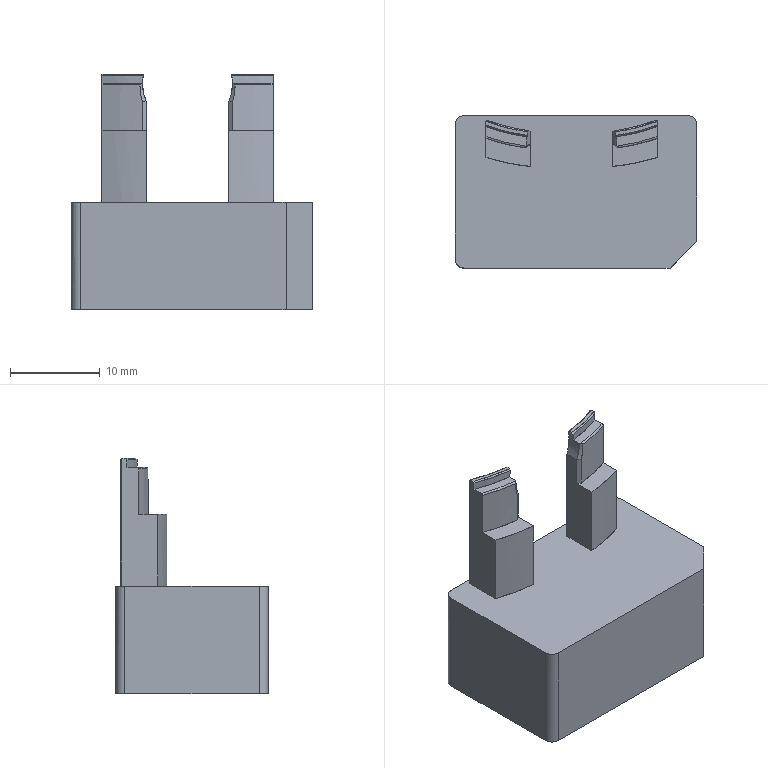NC program | PowerMill | posted by the shop | part box 27 x 17 x 26.255 mm
Lines 17311 to 19049 of 169183:
( TOOL ID   D3_1_1 )
( TOOL DIA. 3. TIP RAD 0 LENGTH 69.4 )
( Z = -14.42 )
T10 M6
T13
G91 G28 Z0
G0 G90 G54
M08
S18000 M3
X0 Y0 M8
G43 Z10.805 H10
X7.533 Y9.349
Z.915
G1 Z-.285 F1200
X7.55 Y9.308 F2000
X7.57 Y9.27
X7.594 Y9.233
X7.621 Y9.199
X7.651 Y9.167
X7.684 Y9.138
X7.72 Y9.112
X7.757 Y9.09
X7.797 Y9.071
X7.838 Y9.056
X7.88 Y9.044
X7.923 Y9.037
X7.966 Y9.033
X8.01
X8.054 Y9.038
X8.097 Y9.046
X8.139 Y9.058
X8.148 Y9.061
X8.39 Y9.149
X8.548 Y9.208
X8.619 Y9.233
X8.691 Y9.254
X8.764 Y9.271
X8.839 Y9.285
X8.913 Y9.294
X8.989 Y9.299
X9.064 Y9.301
X9.139 Y9.298
X9.214 Y9.291
X9.289 Y9.281
X9.363 Y9.266
X9.436 Y9.248
X9.508 Y9.225
X9.579 Y9.199
X9.648 Y9.169
X9.716 Y9.136
X9.782 Y9.099
X9.846 Y9.059
X9.907 Y9.015
X9.966 Y8.968
X10.022 Y8.919
X10.076 Y8.866
X10.127 Y8.81
X10.175 Y8.752
X10.22 Y8.691
X10.261 Y8.628
X10.3 Y8.563
X10.334 Y8.496
X10.365 Y8.427
X10.393 Y8.357
X10.416 Y8.286
X10.436 Y8.213
X10.452 Y8.14
X10.464 Y8.065
X10.472 Y7.991
X10.475 Y7.937
X10.477 Y7.883
Y7.829
X10.478 Y7.775
Y7.717
Y7.638
Y7.584
X10.477 Y7.523
Y7.469
X10.476 Y7.415
X10.475 Y7.361
X10.473 Y7.307
X10.467 Y7.234
X10.456 Y7.162
X10.442 Y7.089
X10.424 Y7.017
X10.401 Y6.945
X10.375 Y6.875
X10.345 Y6.806
X10.312 Y6.738
X10.275 Y6.672
X10.235 Y6.609
X10.191 Y6.547
X10.144 Y6.488
X10.094 Y6.432
X10.041 Y6.378
X9.985 Y6.327
X9.927 Y6.279
X9.866 Y6.234
X9.803 Y6.193
X9.738 Y6.155
X9.671 Y6.12
X9.603 Y6.089
X9.532 Y6.062
X9.26 Y5.963
X8.986 Y5.868
X8.711 Y5.776
X8.435 Y5.688
X8.158 Y5.604
X7.874 Y5.521
X7.589 Y5.443
X7.303 Y5.368
X7.016 Y5.297
X6.729 Y5.229
X6.434 Y5.164
X6.137 Y5.103
X5.838 Y5.046
X5.55 Y4.994
X5.257 Y4.945
X4.946 Y4.897
X4.649 Y4.855
X4.574 Y4.846
X4.498 Y4.841
X4.423 Y4.839
X4.352 Y4.841
X4.282 Y4.846
X4.211 Y4.855
X4.137 Y4.869
X4.064 Y4.886
X3.992 Y4.907
X3.921 Y4.932
X3.851 Y4.961
X3.783 Y4.993
X3.717 Y5.029
X3.652 Y5.068
X3.59 Y5.111
X3.53 Y5.157
X3.473 Y5.206
X3.418 Y5.258
X3.366 Y5.313
X3.317 Y5.37
X3.271 Y5.43
X3.231 Y5.489
X3.193 Y5.552
X3.158 Y5.617
X3.126 Y5.685
X3.097 Y5.757
X3.07 Y5.831
X3.049 Y5.901
X3.032 Y5.971
X3.018 Y6.043
X3.008 Y6.115
X3.002 Y6.186
X2.999 Y6.271
X2.998 Y6.377
Y6.498
X2.999 Y6.683
X3. Y6.748
X3.003 Y6.81
X3.009 Y6.875
X3.021 Y6.945
X3.037 Y7.02
X3.056 Y7.097
X3.079 Y7.171
X3.105 Y7.241
X3.134 Y7.308
X3.166 Y7.373
X3.203 Y7.439
X3.244 Y7.502
X3.288 Y7.564
X3.335 Y7.623
X3.385 Y7.68
X3.438 Y7.734
X3.494 Y7.785
X3.552 Y7.833
X3.612 Y7.877
X3.674 Y7.918
X3.739 Y7.956
X3.805 Y7.991
X3.873 Y8.021
X3.943 Y8.049
X4.015 Y8.073
X4.089 Y8.093
X4.164 Y8.109
X4.241 Y8.122
X4.319 Y8.133
X4.575 Y8.17
X4.849 Y8.214
X5.118 Y8.26
X5.397 Y8.313
X5.664 Y8.367
X5.933 Y8.425
X6.204 Y8.487
X6.472 Y8.553
X6.737 Y8.622
X7.001 Y8.695
X7.265 Y8.772
X7.527 Y8.853
X7.787 Y8.938
X8.046 Y9.026
X8.148 Y9.061
X8.189 Y9.078
X8.228 Y9.098
X8.264 Y9.121
X8.299 Y9.148
X8.331 Y9.178
X8.36 Y9.21
X8.387 Y9.245
X8.409 Y9.283
X8.429 Y9.322
X8.444 Y9.363
X8.456 Y9.405
X8.464 Y9.448
X8.468 Y9.492
Y9.535
X8.464 Y9.579
X8.457 Y9.622
X8.445 Y9.664
X8.442 Y9.673
X7.528 Y9.371 Z-.305
X7.545 Y9.331
X7.565 Y9.292
X7.588 Y9.255
X7.615 Y9.221
X7.645 Y9.189
X7.678 Y9.16
X7.713 Y9.134
X7.75 Y9.111
X7.79 Y9.092
X7.831 Y9.076
X7.873 Y9.065
X7.916 Y9.057
X7.96 Y9.053
X8.003
X8.047 Y9.057
X8.09 Y9.065
X8.132 Y9.077
X8.141 Y9.08
X8.27 Y9.126
X8.348 Y9.155
X8.396 Y9.172
X8.443 Y9.19
X8.491 Y9.209
X8.539 Y9.227
X8.588 Y9.244
X8.636 Y9.26
X8.685 Y9.273
X8.735 Y9.285
X8.785 Y9.296
X8.858 Y9.308
X8.933 Y9.316
X9.008 Y9.32
X9.083
X9.158 Y9.317
X9.233 Y9.309
X9.308 Y9.297
X9.381 Y9.281
X9.454 Y9.262
X9.526 Y9.238
X9.596 Y9.211
X9.665 Y9.181
X9.731 Y9.146
X9.796 Y9.109
X9.859 Y9.067
X9.92 Y9.023
X9.979 Y8.975
X10.034 Y8.925
X10.088 Y8.871
X10.138 Y8.815
X10.185 Y8.756
X10.229 Y8.694
X10.269 Y8.631
X10.306 Y8.565
X10.34 Y8.498
X10.37 Y8.429
X10.396 Y8.359
X10.419 Y8.287
X10.438 Y8.214
X10.453 Y8.138
X10.465 Y8.061
X10.472 Y7.99
X10.476 Y7.912
X10.477 Y7.824
Y7.448
Y7.358
X10.475 Y7.294
X10.47 Y7.24
X10.463 Y7.184
X10.454 Y7.127
X10.438 Y7.052
X10.418 Y6.979
X10.395 Y6.907
X10.368 Y6.837
X10.338 Y6.769
X10.304 Y6.701
X10.266 Y6.636
X10.225 Y6.573
X10.18 Y6.512
X10.133 Y6.453
X10.082 Y6.397
X10.028 Y6.344
X9.972 Y6.294
X9.913 Y6.247
X9.852 Y6.203
X9.788 Y6.162
X9.723 Y6.125
X9.656 Y6.091
X9.588 Y6.062
X9.52 Y6.036
X9.248 Y5.937
X8.973 Y5.842
X8.693 Y5.749
X8.418 Y5.661
X8.141 Y5.577
X7.857 Y5.496
X7.567 Y5.416
X7.303 Y5.347
X7.038 Y5.281
X6.745 Y5.213
X6.451 Y5.148
X6.155 Y5.086
X5.857 Y5.029
X5.557 Y4.975
X5.256 Y4.925
X4.952 Y4.878
X4.707 Y4.843
X4.637 Y4.834
X4.567 Y4.826
X4.496 Y4.821
X4.425 Y4.819
X4.353 Y4.821
X4.279 Y4.827
X4.205 Y4.837
X4.133 Y4.851
X4.061 Y4.868
X3.99 Y4.889
X3.92 Y4.913
X3.851 Y4.942
X3.783 Y4.974
X3.717 Y5.01
X3.653 Y5.05
X3.591 Y5.093
X3.531 Y5.14
X3.473 Y5.189
X3.419 Y5.241
X3.367 Y5.296
X3.319 Y5.354
X3.273 Y5.413
X3.232 Y5.475
X3.193 Y5.539
X3.158 Y5.605
X3.125 Y5.674
X3.097 Y5.743
X3.073 Y5.811
X3.053 Y5.879
X3.038 Y5.946
X3.024 Y6.013
X3.016 Y6.059
X3.01 Y6.106
X3.004 Y6.158
X3. Y6.205
X2.999 Y6.252
X2.998 Y6.648
X3. Y6.736
X3.004 Y6.812
X3.009 Y6.862
X3.016 Y6.912
X3.025 Y6.961
X3.034 Y7.011
X3.045 Y7.06
X3.064 Y7.132
X3.088 Y7.204
X3.115 Y7.275
X3.145 Y7.344
X3.18 Y7.411
X3.217 Y7.476
X3.259 Y7.539
X3.303 Y7.6
X3.351 Y7.658
X3.401 Y7.714
X3.455 Y7.768
X3.511 Y7.818
X3.57 Y7.865
X3.632 Y7.909
X3.695 Y7.949
X3.76 Y7.987
X3.827 Y8.02
X3.896 Y8.05
X3.967 Y8.076
X4.039 Y8.099
X4.113 Y8.118
X4.188 Y8.134
X4.265 Y8.145
X4.531 Y8.184
X4.812 Y8.228
X5.092 Y8.276
X5.368 Y8.327
X5.642 Y8.382
X5.916 Y8.441
X6.189 Y8.504
X6.458 Y8.57
X6.726 Y8.64
X6.992 Y8.714
X7.248 Y8.788
X7.49 Y8.863
X7.754 Y8.947
X7.883 Y8.991
X8.012 Y9.035
X8.141 Y9.08
X8.182 Y9.097
X8.221 Y9.117
X8.257 Y9.141
X8.292 Y9.167
X8.324 Y9.197
X8.353 Y9.23
X8.379 Y9.265
X8.402 Y9.303
X8.421 Y9.342
X8.437 Y9.383
X8.448 Y9.425
X8.456 Y9.468
X8.46 Y9.512
Y9.555
X8.456 Y9.599
X8.448 Y9.642
X8.436 Y9.684
X8.433 Y9.693
X7.522 Y9.393 Z-.325
X7.539 Y9.352
X7.559 Y9.313
X7.582 Y9.276
X7.609 Y9.242
X7.639 Y9.21
X7.671 Y9.18
X7.706 Y9.154
X7.744 Y9.132
X7.783 Y9.112
X7.824 Y9.097
X7.866 Y9.085
X7.909 Y9.077
X7.953 Y9.073
X7.996
X8.04 Y9.077
X8.083 Y9.085
X8.125 Y9.096
X8.134 Y9.1
X8.217 Y9.129
X8.269 Y9.147
X8.314 Y9.164
X8.358 Y9.18
X8.403 Y9.197
X8.447 Y9.213
X8.492 Y9.23
X8.536 Y9.247
X8.582 Y9.263
X8.638 Y9.281
X8.689 Y9.295
X8.735 Y9.306
X8.781 Y9.315
X8.828 Y9.323
X8.875 Y9.329
X8.948 Y9.336
X9.022 Y9.34
X9.096 Y9.339
X9.171 Y9.334
X9.246 Y9.325
X9.32 Y9.312
X9.394 Y9.295
X9.467 Y9.275
X9.538 Y9.25
X9.608 Y9.222
X9.676 Y9.19
X9.743 Y9.155
X9.807 Y9.116
X9.87 Y9.074
X9.93 Y9.029
X9.988 Y8.98
X10.043 Y8.928
X10.095 Y8.874
X10.144 Y8.817
X10.191 Y8.757
X10.234 Y8.696
X10.273 Y8.632
X10.309 Y8.565
X10.343 Y8.496
X10.372 Y8.425
X10.399 Y8.352
X10.421 Y8.278
X10.44 Y8.202
X10.455 Y8.129
X10.466 Y8.055
X10.473 Y7.98
X10.476 Y7.899
X10.477 Y7.814
Y7.348
X10.475 Y7.278
X10.469 Y7.206
X10.459 Y7.133
X10.444 Y7.059
X10.427 Y6.986
X10.405 Y6.913
X10.379 Y6.843
X10.35 Y6.773
X10.317 Y6.705
X10.281 Y6.639
X10.241 Y6.575
X10.198 Y6.513
X10.151 Y6.454
X10.102 Y6.397
X10.049 Y6.343
X9.994 Y6.291
X9.936 Y6.243
X9.876 Y6.198
X9.813 Y6.156
X9.748 Y6.117
X9.681 Y6.082
X9.613 Y6.051
X9.542 Y6.023
X9.265 Y5.922
X8.986 Y5.825
X8.705 Y5.732
X8.421 Y5.642
X8.137 Y5.555
X7.85 Y5.473
X7.561 Y5.394
X7.271 Y5.318
X6.978 Y5.246
X6.684 Y5.178
X6.388 Y5.114
X6.091 Y5.053
X5.791 Y4.996
X5.491 Y4.943
X5.189 Y4.894
X4.927 Y4.854
X4.649 Y4.815
X4.571 Y4.806
X4.494 Y4.801
X4.417 Y4.8
X4.341 Y4.803
X4.266 Y4.81
X4.192 Y4.82
X4.118 Y4.835
X4.046 Y4.854
X3.974 Y4.876
X3.903 Y4.902
X3.834 Y4.932
X3.766 Y4.966
X3.701 Y5.003
X3.637 Y5.044
X3.576 Y5.087
X3.517 Y5.135
X3.46 Y5.185
X3.407 Y5.238
X3.356 Y5.293
X3.308 Y5.352
X3.264 Y5.413
X3.223 Y5.475
X3.185 Y5.54
X3.151 Y5.607
X3.12 Y5.676
X3.092 Y5.747
X3.069 Y5.82
X3.049 Y5.893
X3.032 Y5.968
X3.017 Y6.054
X3.007 Y6.13
X3.001 Y6.198
X2.999 Y6.262
Y6.337
X2.998 Y6.412
Y6.487
Y6.562
Y6.636
X2.999 Y6.711
X3.001 Y6.774
X3.006 Y6.839
X3.016 Y6.911
X3.031 Y6.996
X3.046 Y7.067
X3.064 Y7.138
X3.085 Y7.208
X3.111 Y7.278
X3.141 Y7.347
X3.174 Y7.415
X3.211 Y7.48
X3.252 Y7.544
X3.295 Y7.606
X3.342 Y7.665
X3.392 Y7.721
X3.445 Y7.775
X3.5 Y7.826
X3.559 Y7.874
X3.619 Y7.919
X3.682 Y7.96
X3.747 Y7.998
X3.814 Y8.032
X3.882 Y8.063
X3.953 Y8.091
X4.024 Y8.115
X4.098 Y8.135
X4.172 Y8.151
X4.248 Y8.163
X4.324 Y8.174
X4.598 Y8.214
X4.881 Y8.26
X5.16 Y8.309
X5.434 Y8.361
X5.708 Y8.417
X5.981 Y8.476
X6.253 Y8.54
X6.522 Y8.607
X6.789 Y8.678
X7.054 Y8.752
X7.317 Y8.83
X7.555 Y8.904
X7.759 Y8.97
X7.964 Y9.04
X8.134 Y9.1
X8.175 Y9.116
X8.214 Y9.136
X8.251 Y9.16
X8.285 Y9.186
X8.318 Y9.216
X8.347 Y9.249
X8.373 Y9.284
X8.396 Y9.321
X8.415 Y9.36
X8.431 Y9.401
X8.442 Y9.443
X8.45 Y9.486
X8.454 Y9.53
Y9.574
X8.45 Y9.617
X8.443 Y9.66
X8.431 Y9.703
X8.428 Y9.712
X7.512 Y9.406 Z-.345
X7.529 Y9.365
X7.549 Y9.327
X7.573 Y9.29
X7.6 Y9.256
X7.631 Y9.224
X7.663 Y9.195
X7.699 Y9.169
X7.736 Y9.147
X7.776 Y9.128
X7.817 Y9.113
X7.859 Y9.101
X7.902 Y9.094
X7.946 Y9.09
X7.99 Y9.091
X8.033 Y9.095
X8.076 Y9.104
X8.118 Y9.116
X8.127 Y9.119
X8.136 Y9.122
X8.189 Y9.141
X8.241 Y9.16
X8.294 Y9.179
X8.347 Y9.197
X8.348 Y9.198
X8.401 Y9.217
X8.467 Y9.241
X8.515 Y9.26
X8.574 Y9.281
X8.625 Y9.297
X8.674 Y9.311
X8.723 Y9.323
X8.773 Y9.333
X8.823 Y9.341
X8.874 Y9.348
X8.942 Y9.354
X9.014 Y9.357
X9.088 Y9.356
X9.163 Y9.351
X9.238 Y9.342
X9.312 Y9.329
X9.385 Y9.312
X9.458 Y9.291
X9.529 Y9.267
X9.599 Y9.239
X9.667 Y9.207
X9.734 Y9.171
X9.799 Y9.132
X9.861 Y9.09
X9.921 Y9.044
X9.979 Y8.996
X10.034 Y8.944
X10.086 Y8.89
X10.135 Y8.833
X10.182 Y8.771
X10.226 Y8.708
X10.267 Y8.642
X10.305 Y8.574
X10.339 Y8.504
X10.37 Y8.432
X10.397 Y8.358
X10.42 Y8.284
X10.439 Y8.208
X10.454 Y8.136
X10.465 Y8.064
X10.472 Y7.989
X10.476 Y7.912
X10.477 Y7.838
Y7.353
X10.476 Y7.278
X10.47 Y7.202
X10.461 Y7.127
X10.448 Y7.053
X10.43 Y6.979
X10.409 Y6.906
X10.385 Y6.835
X10.356 Y6.765
X10.324 Y6.697
X10.288 Y6.631
X10.249 Y6.566
X10.206 Y6.504
X10.16 Y6.444
X10.112 Y6.387
X10.06 Y6.332
X10.005 Y6.28
X9.948 Y6.231
X9.888 Y6.185
X9.825 Y6.143
X9.761 Y6.103
X9.695 Y6.068
X9.626 Y6.035
X9.557 Y6.007
X9.486 Y5.981
X9.209 Y5.881
X8.929 Y5.785
X8.648 Y5.692
X8.364 Y5.603
X8.078 Y5.518
X7.792 Y5.436
X7.503 Y5.358
X7.212 Y5.283
X6.918 Y5.212
X6.627 Y5.145
X6.332 Y5.082
X6.034 Y5.022
X5.731 Y4.965
X5.455 Y4.917
X5.165 Y4.87
X4.849 Y4.823
X4.649 Y4.795
X4.57 Y4.786
X4.493 Y4.781
X4.416 Y4.78
X4.339 Y4.784
X4.264 Y4.791
X4.19 Y4.802
X4.118 Y4.816
X4.046 Y4.835
X3.974 Y4.858
X3.903 Y4.884
X3.834 Y4.914
X3.767 Y4.948
X3.701 Y4.986
X3.637 Y5.027
X3.576 Y5.071
X3.517 Y5.118
X3.461 Y5.168
X3.407 Y5.221
X3.357 Y5.277
X3.31 Y5.334
X3.266 Y5.395
X3.225 Y5.458
X3.186 Y5.525
X3.15 Y5.595
X3.123 Y5.655
X3.099 Y5.719
X3.077 Y5.788
X3.056 Y5.865
X3.037 Y5.948
X3.02 Y6.029
X3.011 Y6.089
X3.005 Y6.14
X3.003 Y6.189
X2.999 Y6.297
X2.998 Y6.394
Y6.498
Y6.617
Y6.704
X3.002 Y6.78
X3.009 Y6.863
X3.021 Y6.947
X3.037 Y7.03
X3.056 Y7.113
X3.076 Y7.186
X3.097 Y7.252
X3.124 Y7.321
X3.154 Y7.389
X3.188 Y7.455
X3.225 Y7.517
X3.264 Y7.578
X3.31 Y7.64
X3.359 Y7.7
X3.409 Y7.756
X3.463 Y7.809
X3.518 Y7.859
X3.576 Y7.905
X3.636 Y7.948
X3.7 Y7.99
X3.766 Y8.027
X3.834 Y8.061
X3.903 Y8.091
X3.974 Y8.118
X4.045 Y8.14
X4.11 Y8.157
X4.175 Y8.171
X4.241 Y8.182
X4.307 Y8.192
X4.373 Y8.201
X4.439 Y8.211
X4.505 Y8.22
X4.571 Y8.23
X4.637 Y8.241
X4.703 Y8.251
X4.988 Y8.298
X5.264 Y8.348
X5.531 Y8.4
X5.796 Y8.456
X6.07 Y8.517
X6.341 Y8.582
X6.605 Y8.649
X6.868 Y8.72
X7.13 Y8.795
X7.398 Y8.876
X7.575 Y8.932
X7.796 Y9.003
X7.849 Y9.02
X7.902 Y9.038
X7.955 Y9.056
X8.007 Y9.075
X8.061 Y9.095
X8.127 Y9.119
X8.168 Y9.136
X8.206 Y9.156
X8.243 Y9.18
X8.278 Y9.207
X8.309 Y9.237
X8.338 Y9.27
X8.364 Y9.306
X8.386 Y9.343
X8.405 Y9.383
X8.42 Y9.424
X8.432 Y9.466
X8.439 Y9.509
X8.443 Y9.553
X8.442 Y9.596
X8.438 Y9.64
X8.43 Y9.683
X8.418 Y9.725
X8.414 Y9.734
X7.507 Y9.428 Z-.365
X7.524 Y9.387
X7.544 Y9.348
X7.568 Y9.311
X7.595 Y9.277
X7.625 Y9.245
X7.658 Y9.216
X7.693 Y9.19
X7.73 Y9.167
X7.77 Y9.148
X7.81 Y9.133
X7.853 Y9.121
X7.896 Y9.113
X7.939 Y9.109
X7.983 Y9.11
X8.027 Y9.114
X8.07 Y9.122
X8.112 Y9.134
X8.121 Y9.137
X8.248 Y9.182
X8.348 Y9.219
X8.483 Y9.269
X8.574 Y9.301
X8.651 Y9.324
X8.719 Y9.342
X8.783 Y9.355
X8.842 Y9.363
X8.903 Y9.369
X8.981 Y9.372
X9.059 Y9.371
X9.137 Y9.367
X9.214 Y9.358
X9.287 Y9.347
X9.359 Y9.331
X9.43 Y9.311
X9.501 Y9.288
X9.57 Y9.261
X9.639 Y9.23
X9.705 Y9.195
X9.77 Y9.157
X9.833 Y9.115
X9.894 Y9.07
X9.953 Y9.021
X10.01 Y8.968
X10.065 Y8.913
X10.117 Y8.854
X10.166 Y8.793
X10.212 Y8.73
X10.254 Y8.664
X10.293 Y8.597
X10.328 Y8.527
X10.36 Y8.456
X10.388 Y8.383
X10.412 Y8.309
X10.433 Y8.234
X10.447 Y8.171
X10.46 Y8.097
X10.469 Y8.03
X10.473 Y7.969
X10.474 Y7.909
X10.477 Y7.638
X10.478 Y7.348
X10.476 Y7.265
X10.47 Y7.186
X10.462 Y7.112
X10.45 Y7.041
X10.433 Y6.967
X10.412 Y6.895
X10.388 Y6.823
X10.36 Y6.753
X10.328 Y6.685
X10.293 Y6.618
X10.254 Y6.553
X10.212 Y6.491
X10.167 Y6.43
X10.118 Y6.373
X10.067 Y6.318
X10.012 Y6.265
X9.955 Y6.216
X9.896 Y6.17
X9.834 Y6.127
X9.77 Y6.087
X9.703 Y6.051
X9.636 Y6.018
X9.566 Y5.989
X9.495 Y5.963
X9.219 Y5.863
X8.94 Y5.767
X8.658 Y5.675
X8.374 Y5.585
X8.088 Y5.5
X7.801 Y5.418
X7.512 Y5.339
X7.221 Y5.265
X6.928 Y5.193
X6.633 Y5.126
X6.337 Y5.062
X6.038 Y5.002
X5.74 Y4.946
X5.439 Y4.894
X5.154 Y4.848
X4.848 Y4.802
X4.649 Y4.775
X4.571 Y4.766
X4.494 Y4.761
X4.417
X4.342 Y4.764
X4.268 Y4.771
X4.195 Y4.782
X4.121 Y4.797
X4.048 Y4.816
X3.976 Y4.839
X3.905 Y4.865
X3.836 Y4.896
X3.769 Y4.93
X3.703 Y4.967
X3.64 Y5.008
X3.579 Y5.052
X3.52 Y5.099
X3.464 Y5.149
X3.41 Y5.203
X3.36 Y5.259
X3.312 Y5.318
X3.269 Y5.377
X3.228 Y5.439
X3.19 Y5.505
X3.154 Y5.575
X3.128 Y5.633
X3.104 Y5.695
X3.082 Y5.764
X3.059 Y5.845
X3.049 Y5.886
X3.042 Y5.919
X3.035 Y5.953
X3.028 Y5.988
X3.018 Y6.043
X3.013 Y6.077
X3.009 Y6.11
X3.005 Y6.144
X3.003 Y6.179
X2.999 Y6.288
X2.998 Y6.385
Y6.609
X2.999 Y6.733
X3.002 Y6.791
X3.008 Y6.855
X3.019 Y6.929
X3.037 Y7.029
X3.052 Y7.104
X3.071 Y7.178
X3.093 Y7.249
X3.119 Y7.32
X3.149 Y7.388
X3.182 Y7.456
X3.219 Y7.522
X3.259 Y7.586
X3.303 Y7.647
X3.35 Y7.706
X3.4 Y7.763
X3.453 Y7.817
X3.508 Y7.868
X3.567 Y7.916
X3.627 Y7.96
X3.69 Y8.002
X3.755 Y8.04
X3.822 Y8.074
X3.891 Y8.106
X3.962 Y8.133
X4.033 Y8.157
X4.107 Y8.176
X4.181 Y8.192
X4.255 Y8.204
X4.551 Y8.247
X4.842 Y8.294
X5.12 Y8.342
X5.397 Y8.394
X5.672 Y8.45
X5.945 Y8.509
X6.216 Y8.572
X6.485 Y8.639
X6.752 Y8.709
X7.017 Y8.783
X7.28 Y8.86
X7.54 Y8.941
X7.799 Y9.026
X8.055 Y9.113
X8.121 Y9.137
X8.161 Y9.154
X8.2 Y9.174
X8.237 Y9.197
X8.272 Y9.224
X8.304 Y9.254
X8.333 Y9.287
X8.359 Y9.322
X8.381 Y9.36
X8.4 Y9.399
X8.416 Y9.44
X8.427 Y9.482
X8.435 Y9.525
X8.439 Y9.569
Y9.613
X8.435 Y9.656
X8.427 Y9.699
X8.415 Y9.741
X8.412 Y9.75
X7.501 Y9.447 Z-.385
X7.518 Y9.407
X7.538 Y9.368
X7.562 Y9.331
X7.588 Y9.297
X7.618 Y9.265
X7.651 Y9.236
X7.686 Y9.21
X7.724 Y9.187
X7.763 Y9.168
X7.804 Y9.152
X7.846 Y9.14
X7.889 Y9.132
X7.933 Y9.129
X7.976
X8.02 Y9.133
X8.063 Y9.141
X8.105 Y9.153
X8.114 Y9.156
X8.248 Y9.203
X8.303 Y9.224
X8.357 Y9.244
X8.412 Y9.265
X8.482 Y9.29
X8.537 Y9.31
X8.592 Y9.327
X8.648 Y9.343
X8.716 Y9.359
X8.789 Y9.371
X8.863 Y9.38
X8.937 Y9.385
X9.011 Y9.386
X9.086 Y9.384
X9.16 Y9.377
X9.234 Y9.366
X9.308 Y9.351
X9.381 Y9.333
X9.453 Y9.31
X9.524 Y9.284
X9.594 Y9.254
X9.662 Y9.22
X9.73 Y9.182
X9.796 Y9.141
X9.86 Y9.096
X9.921 Y9.048
X9.98 Y8.997
X10.036 Y8.943
X10.09 Y8.886
X10.14 Y8.826
X10.188 Y8.764
X10.232 Y8.7
X10.272 Y8.633
X10.31 Y8.565
X10.343 Y8.495
X10.373 Y8.423
X10.4 Y8.349
X10.422 Y8.275
X10.441 Y8.199
X10.455 Y8.127
X10.466 Y8.054
X10.473 Y7.979
X10.476 Y7.902
X10.477 Y7.828
Y7.474
X10.478 Y7.348
X10.477 Y7.273
X10.473 Y7.196
X10.466 Y7.121
X10.455 Y7.05
X10.441 Y6.981
X10.424 Y6.913
X10.402 Y6.841
X10.376 Y6.77
X10.346 Y6.701
X10.313 Y6.634
X10.276 Y6.568
X10.236 Y6.504
X10.192 Y6.442
X10.146 Y6.383
X10.096 Y6.327
X10.043 Y6.273
X9.988 Y6.222
X9.929 Y6.174
X9.869 Y6.129
X9.806 Y6.088
X9.741 Y6.049
X9.674 Y6.015
X9.605 Y5.984
X9.535 Y5.956
X9.263 Y5.858
X8.989 Y5.763
X8.713 Y5.671
X8.432 Y5.582
X8.146 Y5.496
X7.858 Y5.413
X7.57 Y5.334
X7.283 Y5.259
X6.997 Y5.189
X6.701 Y5.121
X6.404 Y5.056
X6.105 Y4.995
X5.809 Y4.938
X5.512 Y4.886
X5.21 Y4.836
X4.904 Y4.79
X4.649 Y4.755
X4.569 Y4.746
X4.492 Y4.742
X4.416 Y4.741
X4.342 Y4.744
X4.27 Y4.751
X4.199 Y4.762
X4.124 Y4.777
X4.051 Y4.797
X3.979 Y4.819
X3.908 Y4.846
X3.839 Y4.876
X3.772 Y4.91
X3.709 Y4.946
X3.647 Y4.986
X3.584 Y5.031
X3.528 Y5.076
X3.473 Y5.124
X3.42 Y5.176
X3.37 Y5.231
X3.323 Y5.289
X3.278 Y5.35
X3.235 Y5.414
X3.198 Y5.477
X3.167 Y5.537
X3.144 Y5.587
X3.122 Y5.638
X3.103 Y5.689
X3.085 Y5.742
X3.071 Y5.795
X3.058 Y5.849
X3.049 Y5.884
X3.041 Y5.92
X3.034 Y5.956
X3.028 Y5.993
X3.018 Y6.05
X3.012 Y6.087
X3.008 Y6.123
X3.004 Y6.16
X3. Y6.242
X2.998 Y6.342
Y6.485
X2.999 Y6.654
X3. Y6.748
X3.002 Y6.795
X3.007 Y6.846
X3.015 Y6.902
X3.023 Y6.949
X3.036 Y7.031
X3.048 Y7.087
X3.061 Y7.142
X3.084 Y7.225
X3.107 Y7.296
X3.129 Y7.357
X3.156 Y7.417
X3.188 Y7.481
X3.226 Y7.548
X3.265 Y7.61
X3.308 Y7.669
X3.354 Y7.727
X3.404 Y7.784
X3.455 Y7.836
X3.509 Y7.885
X3.566 Y7.933
X3.626 Y7.978
X3.689 Y8.019
X3.754 Y8.058
X3.821 Y8.093
X3.889 Y8.124
X3.959 Y8.151
X4.031 Y8.175
X4.103 Y8.195
X4.177 Y8.212
X4.252 Y8.224
X4.556 Y8.268
X4.838 Y8.313
X5.107 Y8.36
X5.385 Y8.412
X5.659 Y8.468
X5.932 Y8.527
X6.201 Y8.589
X6.469 Y8.656
X6.737 Y8.726
X7.004 Y8.8
X7.258 Y8.875
X7.513 Y8.954
X7.772 Y9.038
X8.035 Y9.128
X8.114 Y9.156
X8.155 Y9.172
X8.194 Y9.192
X8.231 Y9.216
X8.265 Y9.243
X8.297 Y9.273
X8.326 Y9.305
X8.352 Y9.341
X8.375 Y9.378
X8.394 Y9.417
X8.41 Y9.458
X8.421 Y9.5
X8.429 Y9.543
X8.433 Y9.587
Y9.631
X8.429 Y9.674
X8.421 Y9.717
X8.409 Y9.759
X8.406 Y9.769
X7.495 Y9.467 Z-.405
X7.512 Y9.426
X7.532 Y9.388
X7.555 Y9.351
X7.582 Y9.316
X7.612 Y9.284
X7.644 Y9.255
X7.68 Y9.229
X7.717 Y9.206
X7.756 Y9.187
X7.797 Y9.171
X7.839 Y9.159
X7.882 Y9.151
X7.926 Y9.147
X7.97
X8.013 Y9.151
X8.056 Y9.159
X8.098 Y9.171
X8.108 Y9.174
X8.148 Y9.189
X8.189 Y9.204
X8.23 Y9.219
X8.271 Y9.234
X8.323 Y9.254
X8.402 Y9.283
X8.458 Y9.303
X8.5 Y9.318
X8.542 Y9.332
X8.583 Y9.345
X8.626 Y9.355
X8.702 Y9.371
X8.779 Y9.383
X8.854 Y9.391
X8.93 Y9.394
X9.004
X9.079 Y9.39
X9.155 Y9.382
X9.231 Y9.37
X9.307 Y9.354
X9.383 Y9.333
X9.457 Y9.309
X9.531 Y9.282
X9.602 Y9.25
X9.672 Y9.215
X9.739 Y9.177
X9.805 Y9.135
X9.868 Y9.09
X9.929 Y9.042
X9.988 Y8.99
X10.044 Y8.935
X10.097 Y8.878
X10.147 Y8.818
X10.194 Y8.755
X10.238 Y8.691
X10.278 Y8.624
X10.314 Y8.556
X10.348 Y8.485
X10.377 Y8.413
X10.403 Y8.339
X10.425 Y8.264
X10.443 Y8.188
X10.457 Y8.116
X10.467 Y8.043
X10.474 Y7.967
X10.477 Y7.89
Y7.815
X10.476 Y7.248
X10.474 Y7.182
X10.468 Y7.116
X10.458 Y7.046
X10.444 Y6.973
X10.426 Y6.899
X10.404 Y6.826
X10.378 Y6.755
X10.35 Y6.688
X10.32 Y6.625
X10.283 Y6.558
X10.244 Y6.494
X10.201 Y6.432
X10.154 Y6.373
X10.105 Y6.315
X10.052 Y6.261
X9.997 Y6.209
X9.94 Y6.161
X9.879 Y6.115
X9.817 Y6.073
X9.753 Y6.035
X9.686 Y5.999
X9.618 Y5.968
X9.548 Y5.94
X9.477 Y5.914
X9.201 Y5.815
X8.923 Y5.719
X8.642 Y5.627
X8.359 Y5.539
X8.073 Y5.453
X7.785 Y5.372
X7.494 Y5.293
X7.201 Y5.218
X6.912 Y5.148
X6.623 Y5.083
X6.33 Y5.02
X6.032 Y4.96
X5.741 Y4.906
X5.446 Y4.854
X5.14 Y4.805
X4.824 Y4.758
X4.649 Y4.734
X4.573 Y4.726
X4.497 Y4.721
X4.421
X4.345 Y4.725
X4.269 Y4.732
X4.194 Y4.744
X4.121 Y4.759
X4.048 Y4.779
X3.976 Y4.802
X3.906 Y4.829
X3.837 Y4.859
X3.77 Y4.894
X3.704 Y4.931
X3.641 Y4.972
X3.58 Y5.017
X3.522 Y5.064
X3.466 Y5.115
X3.413 Y5.168
X3.363 Y5.224
X3.316 Y5.283
X3.271 Y5.345
X3.231 Y5.408
X3.193 Y5.474
X3.159 Y5.541
X3.13 Y5.609
X3.104 Y5.678
X3.081 Y5.75
X3.062 Y5.825
X3.049 Y5.884
X3.043 Y5.914
X3.037 Y5.943
X3.031 Y5.975
X3.023 Y6.021
X3.018 Y6.051
X3.012 Y6.087
X3.008 Y6.117
X3.005 Y6.147
X3.004 Y6.177
X2.999 Y6.286
X2.998 Y6.377
Y6.498
Y6.651
X3. Y6.748
X3.004 Y6.81
X3.012 Y6.88
X3.025 Y6.962
X3.045 Y7.07
X3.06 Y7.144
X3.079 Y7.216
X3.101 Y7.287
X3.127 Y7.356
X3.158 Y7.425
X3.192 Y7.493
X3.229 Y7.558
X3.27 Y7.622
X3.314 Y7.683
X3.36 Y7.741
X3.41 Y7.797
X3.463 Y7.85
X3.519 Y7.901
X3.578 Y7.949
X3.64 Y7.994
X3.703 Y8.035
X3.768 Y8.073
X3.835 Y8.107
X3.903 Y8.137
X3.973 Y8.164
X4.043 Y8.186
X4.114 Y8.205
X4.186 Y8.22
X4.371 Y8.256
X4.568 Y8.29
X4.873 Y8.34
X5.091 Y8.377
X5.369 Y8.429
X5.644 Y8.485
X5.917 Y8.544
X6.188 Y8.607
X6.455 Y8.673
X6.722 Y8.742
X6.987 Y8.816
X7.25 Y8.893
X7.512 Y8.974
X7.771 Y9.059
X8.029 Y9.147
X8.108 Y9.174
X8.148 Y9.191
X8.187 Y9.211
X8.224 Y9.234
X8.259 Y9.261
X8.291 Y9.291
X8.32 Y9.324
X8.346 Y9.359
X8.369 Y9.396
X8.388 Y9.436
X8.404 Y9.476
X8.415 Y9.519
X8.423 Y9.562
X8.427 Y9.605
Y9.649
X8.423 Y9.693
X8.415 Y9.736
X8.403 Y9.778
X8.4 Y9.787
X7.491 Y9.477 Z-.425
X7.508 Y9.437
X7.528 Y9.398
X7.551 Y9.361
X7.578 Y9.326
X7.608 Y9.294
X7.641 Y9.265
X7.676 Y9.239
X7.713 Y9.217
X7.752 Y9.197
X7.793 Y9.182
X7.835 Y9.17
X7.878 Y9.162
X7.922 Y9.158
X7.966
X8.009 Y9.162
X8.052 Y9.17
X8.095 Y9.182
X8.104 Y9.185
X8.136 Y9.197
X8.412 Y9.297
X8.479 Y9.321
X8.549 Y9.342
X8.622 Y9.36
X8.699 Y9.374
X8.776 Y9.385
X8.853 Y9.392
X8.93 Y9.396
X9.008 Y9.395
X9.085 Y9.39
X9.163 Y9.381
X9.24 Y9.368
X9.316 Y9.351
X9.391 Y9.331
X9.465 Y9.307
X9.538 Y9.278
X9.609 Y9.247
X9.679 Y9.211
X9.747 Y9.172
X9.812 Y9.13
X9.875 Y9.085
X9.936 Y9.036
X9.994 Y8.984
X10.05 Y8.929
X10.103 Y8.871
X10.152 Y8.811
X10.199 Y8.748
X10.242 Y8.683
X10.282 Y8.617
X10.318 Y8.548
X10.351 Y8.477
X10.38 Y8.405
X10.406 Y8.331
X10.427 Y8.256
X10.445 Y8.179
X10.458 Y8.108
X10.468 Y8.035
X10.474 Y7.958
X10.477 Y7.881
Y7.804
Y7.248
X10.475 Y7.179
X10.469 Y7.109
X10.459 Y7.037
X10.445 Y6.964
X10.427 Y6.89
X10.405 Y6.817
X10.379 Y6.745
X10.349 Y6.674
X10.316 Y6.606
X10.281 Y6.541
X10.242 Y6.48
X10.201 Y6.421
X10.155 Y6.361
X10.105 Y6.304
X10.052 Y6.249
X9.997 Y6.198
X9.939 Y6.149
X9.879 Y6.103
X9.816 Y6.061
X9.752 Y6.023
X9.685 Y5.988
X9.617 Y5.956
X9.547 Y5.928
X9.477 Y5.902
X9.201 Y5.803
X8.923 Y5.708
X8.642 Y5.616
X8.358 Y5.527
X8.072 Y5.442
X7.784 Y5.36
X7.494 Y5.282
X7.202 Y5.208
X6.911 Y5.137
X6.616 Y5.07
X6.318 Y5.007
X6.017 Y4.946
X5.731 Y4.893
X5.437 Y4.842
X5.133 Y4.793
X4.817 Y4.747
X4.649 Y4.723
X4.573 Y4.715
X4.497 Y4.711
X4.421
X4.346 Y4.714
X4.27 Y4.722
X4.195 Y4.734
X4.121 Y4.749
X4.049 Y4.769
X3.977 Y4.792
X3.907 Y4.819
X3.838 Y4.849
X3.771 Y4.883
X3.706 Y4.921
X3.643 Y4.962
X3.582 Y5.006
X3.524 Y5.054
X3.468 Y5.104
X3.415 Y5.158
X3.365 Y5.214
X3.318 Y5.273
X3.274 Y5.335
X3.233 Y5.399
X3.195 Y5.465
X3.161 Y5.533
X3.133 Y5.595
X3.109 Y5.658
X3.088 Y5.722
X3.074 Y5.773
X3.059 Y5.838
X3.051 Y5.872
X3.044 Y5.906
X3.037 Y5.94
X3.029 Y5.983
X3.02 Y6.04
X3.014 Y6.077
X3.009 Y6.112
X3.005 Y6.146
X3.003 Y6.181
X2.999 Y6.268
X2.998 Y6.375
Y6.498
X2.999 Y6.689
X3. Y6.748
X3.002 Y6.794
X3.007 Y6.844
X3.015 Y6.899
X3.022 Y6.945
X3.03 Y6.991
X3.039 Y7.047
X3.052 Y7.103
X3.066 Y7.164
X3.082 Y7.225
X3.1 Y7.285
X3.125 Y7.351
X3.154 Y7.418
X3.187 Y7.484
X3.225 Y7.55
X3.266 Y7.615
X3.31 Y7.677
X3.357 Y7.736
X3.407 Y7.793
X3.457 Y7.844
X3.51 Y7.893
X3.567 Y7.94
X3.627 Y7.985
X3.69 Y8.027
X3.756 Y8.066
X3.823 Y8.101
X3.891 Y8.132
X3.959 Y8.159
X4.027 Y8.182
X4.095 Y8.201
X4.163 Y8.215
X4.447 Y8.27
X4.731 Y8.322
X5.015 Y8.374
X5.277 Y8.423
X5.563 Y8.479
X5.84 Y8.538
X6.11 Y8.6
X6.373 Y8.663
X6.631 Y8.73
X6.888 Y8.799
X7.144 Y8.873
X7.401 Y8.951
X7.655 Y9.032
X7.907 Y9.116
X7.948 Y9.13
X8.104 Y9.185
X8.144 Y9.202
X8.183 Y9.222
X8.22 Y9.246
X8.255 Y9.272
X8.287 Y9.302
X8.316 Y9.335
X8.342 Y9.37
X8.365 Y9.407
X8.384 Y9.447
X8.399 Y9.488
X8.411 Y9.53
X8.419 Y9.573
X8.423 Y9.616
Y9.66
X8.419 Y9.704
X8.411 Y9.747
X8.399 Y9.789
X8.396 Y9.798
X7.49 Y9.475 Z-.475
X7.507 Y9.435
X7.527 Y9.396
X7.551 Y9.359
X7.578 Y9.325
X7.608 Y9.293
X7.64 Y9.264
X7.676 Y9.238
X7.713 Y9.215
X7.752 Y9.196
X7.793 Y9.181
X7.835 Y9.169
X7.879 Y9.161
X7.922 Y9.158
X7.966
X8.009 Y9.162
X8.052 Y9.17
X8.094 Y9.182
X8.104 Y9.185
X8.195 Y9.218
X8.248 Y9.236
X8.341 Y9.27
X8.446 Y9.308
X8.523 Y9.334
X8.584 Y9.351
X8.649 Y9.366
X8.723 Y9.378
X8.799 Y9.388
X8.876 Y9.394
X8.954 Y9.396
X9.031 Y9.394
X9.109 Y9.388
X9.187 Y9.377
X9.264 Y9.363
X9.339 Y9.346
X9.414 Y9.324
X9.488 Y9.298
X9.56 Y9.269
X9.631 Y9.236
X9.7 Y9.2
X9.767 Y9.16
X9.832 Y9.116
X9.894 Y9.07
X9.954 Y9.02
X10.012 Y8.967
X10.067 Y8.911
X10.118 Y8.853